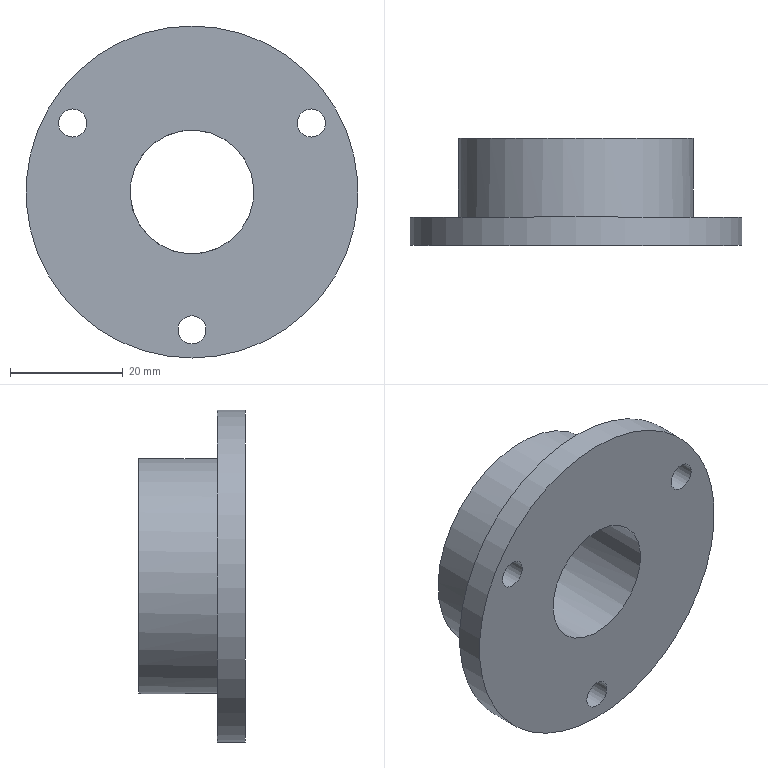Part | STEP file | YBQDJ-YB-12 | 1 solid | 11 faces | box 59 x 19 x 59 mm | volume 24092 mm3 | cylinder 7 | plane 4 | commonest cylinder face diameters 5 x3 22 x1 32 x1 41.8 x1 59 x1
STEP:
#1=CARTESIAN_POINT('',(0.,0.,0.));
#2=DIRECTION('',(0.,0.,1.));
#3=DIRECTION('',(1.,0.,0.));
#4=AXIS2_PLACEMENT_3D('',#1,#2,#3);
#5=CARTESIAN_POINT('',(-168.721,-300.,118.779));
#6=VERTEX_POINT('',#5);
#7=CARTESIAN_POINT('',(-183.5,-300.,104.));
#8=DIRECTION('',(0.,1.,0.));
#9=DIRECTION('',(0.7071,0.,0.7071));
#10=AXIS2_PLACEMENT_3D('',#7,#8,#9);
#11=CIRCLE('',#10,20.9);
#12=CARTESIAN_POINT('',(-183.5,-295.,104.));
#13=DIRECTION('',(0.,-1.,0.));
#14=DIRECTION('',(0.7071,0.,0.7071));
#15=AXIS2_PLACEMENT_3D('',#12,#13,#14);
#16=CYLINDRICAL_SURFACE('',#15,20.9);
#17=CARTESIAN_POINT('',(6.283,5.));
#18=DIRECTION('',(-1.,0.));
#19=VECTOR('',#18,1.);
#20=LINE('',#17,#19);
#21=(GEOMETRIC_REPRESENTATION_CONTEXT(2)PARAMETRIC_REPRESENTATION_CONTEXT()REPRESENTATION_CONTEXT('',''));
#22=DEFINITIONAL_REPRESENTATION('',(#20),#21);
#23=PCURVE('',#16,#22);
#24=CARTESIAN_POINT('',(-183.5,-300.,104.));
#25=DIRECTION('',(0.,1.,0.));
#26=DIRECTION('',(-0.7071,0.,-0.7071));
#27=AXIS2_PLACEMENT_3D('',#24,#25,#26);
#28=PLANE('',#27);
#29=CARTESIAN_POINT('',(0.,0.));
#30=DIRECTION('',(-1.,0.));
#31=AXIS2_PLACEMENT_2D('',#29,#30);
#32=CIRCLE('',#31,20.9);
#33=(GEOMETRIC_REPRESENTATION_CONTEXT(2)PARAMETRIC_REPRESENTATION_CONTEXT()REPRESENTATION_CONTEXT('',''));
#34=DEFINITIONAL_REPRESENTATION('',(#32),#33);
#35=PCURVE('',#28,#34);
#36=SURFACE_CURVE('',#11,(#23,#35),.PCURVE_S1.);
#37=EDGE_CURVE('',#6,#6,#36,.T.);
#38=ORIENTED_EDGE('',*,*,#37,.T.);
#39=CARTESIAN_POINT('',(-168.721,-286.,118.779));
#40=VERTEX_POINT('',#39);
#41=CARTESIAN_POINT('',(-168.721,-286.,118.779));
#42=CARTESIAN_POINT('',(-168.721,-300.,118.779));
#43=B_SPLINE_CURVE_WITH_KNOTS('',1,(#41,#42),.UNSPECIFIED.,.F.,.F.,(2,2),(-9.,5.),.PIECEWISE_BEZIER_KNOTS.);
#44=CARTESIAN_POINT('',(0.,0.));
#45=DIRECTION('',(0.,1.));
#46=VECTOR('',#45,1.);
#47=LINE('',#44,#46);
#48=(GEOMETRIC_REPRESENTATION_CONTEXT(2)PARAMETRIC_REPRESENTATION_CONTEXT()REPRESENTATION_CONTEXT('',''));
#49=DEFINITIONAL_REPRESENTATION('',(#47),#48);
#50=PCURVE('',#16,#49);
#51=CARTESIAN_POINT('',(6.283,0.));
#52=DIRECTION('',(0.,1.));
#53=VECTOR('',#52,1.);
#54=LINE('',#51,#53);
#55=(GEOMETRIC_REPRESENTATION_CONTEXT(2)PARAMETRIC_REPRESENTATION_CONTEXT()REPRESENTATION_CONTEXT('',''));
#56=DEFINITIONAL_REPRESENTATION('',(#54),#55);
#57=PCURVE('',#16,#56);
#58=SEAM_CURVE('',#43,(#50,#57),.PCURVE_S1.);
#59=EDGE_CURVE('',#40,#6,#58,.T.);
#60=ORIENTED_EDGE('',*,*,#59,.F.);
#61=CARTESIAN_POINT('',(-183.5,-286.,83.1));
#62=VERTEX_POINT('',#61);
#63=CARTESIAN_POINT('',(-183.5,-286.,104.));
#64=DIRECTION('',(0.,-1.,0.));
#65=DIRECTION('',(0.,0.,-1.));
#66=AXIS2_PLACEMENT_3D('',#63,#64,#65);
#67=CIRCLE('',#66,20.9);
#68=CARTESIAN_POINT('',(-2.356,-9.));
#69=DIRECTION('',(1.,0.));
#70=VECTOR('',#69,1.);
#71=LINE('',#68,#70);
#72=(GEOMETRIC_REPRESENTATION_CONTEXT(2)PARAMETRIC_REPRESENTATION_CONTEXT()REPRESENTATION_CONTEXT('',''));
#73=DEFINITIONAL_REPRESENTATION('',(#71),#72);
#74=PCURVE('',#16,#73);
#75=CARTESIAN_POINT('',(-183.5,-286.,94.));
#76=DIRECTION('',(0.,-1.,0.));
#77=DIRECTION('',(0.,0.,1.));
#78=AXIS2_PLACEMENT_3D('',#75,#76,#77);
#79=PLANE('',#78);
#80=CARTESIAN_POINT('',(10.,0.));
#81=DIRECTION('',(-1.,0.));
#82=AXIS2_PLACEMENT_2D('',#80,#81);
#83=CIRCLE('',#82,20.9);
#84=(GEOMETRIC_REPRESENTATION_CONTEXT(2)PARAMETRIC_REPRESENTATION_CONTEXT()REPRESENTATION_CONTEXT('',''));
#85=DEFINITIONAL_REPRESENTATION('',(#83),#84);
#86=PCURVE('',#79,#85);
#87=SURFACE_CURVE('',#67,(#74,#86),.PCURVE_S1.);
#88=EDGE_CURVE('',#40,#62,#87,.T.);
#89=ORIENTED_EDGE('',*,*,#88,.T.);
#90=CARTESIAN_POINT('',(-183.5,-286.,104.));
#91=DIRECTION('',(0.,-1.,0.));
#92=DIRECTION('',(0.,0.,-1.));
#93=AXIS2_PLACEMENT_3D('',#90,#91,#92);
#94=CIRCLE('',#93,20.9);
#95=CARTESIAN_POINT('',(3.927,-9.));
#96=DIRECTION('',(1.,0.));
#97=VECTOR('',#96,1.);
#98=LINE('',#95,#97);
#99=(GEOMETRIC_REPRESENTATION_CONTEXT(2)PARAMETRIC_REPRESENTATION_CONTEXT()REPRESENTATION_CONTEXT('',''));
#100=DEFINITIONAL_REPRESENTATION('',(#98),#99);
#101=PCURVE('',#16,#100);
#102=CARTESIAN_POINT('',(10.,0.));
#103=DIRECTION('',(-1.,0.));
#104=AXIS2_PLACEMENT_2D('',#102,#103);
#105=CIRCLE('',#104,20.9);
#106=(GEOMETRIC_REPRESENTATION_CONTEXT(2)PARAMETRIC_REPRESENTATION_CONTEXT()REPRESENTATION_CONTEXT('',''));
#107=DEFINITIONAL_REPRESENTATION('',(#105),#106);
#108=PCURVE('',#79,#107);
#109=SURFACE_CURVE('',#94,(#101,#108),.PCURVE_S1.);
#110=EDGE_CURVE('',#62,#40,#109,.T.);
#111=ORIENTED_EDGE('',*,*,#110,.T.);
#112=ORIENTED_EDGE('',*,*,#59,.T.);
#113=EDGE_LOOP('',(#38,#60,#89,#111,#112));
#114=FACE_BOUND('',#113,.T.);
#115=ADVANCED_FACE('',(#114),#16,.T.);
#116=CARTESIAN_POINT('',(-183.5,-305.,133.5));
#117=VERTEX_POINT('',#116);
#118=CARTESIAN_POINT('',(-183.5,-305.,104.));
#119=DIRECTION('',(0.,-1.,0.));
#120=DIRECTION('',(0.,0.,1.));
#121=AXIS2_PLACEMENT_3D('',#118,#119,#120);
#122=CIRCLE('',#121,29.5);
#123=CARTESIAN_POINT('',(-183.5,-305.,104.));
#124=DIRECTION('',(0.,1.,0.));
#125=DIRECTION('',(-0.7071,0.,-0.7071));
#126=AXIS2_PLACEMENT_3D('',#123,#124,#125);
#127=CYLINDRICAL_SURFACE('',#126,29.5);
#128=CARTESIAN_POINT('',(8.639,0.));
#129=DIRECTION('',(-1.,0.));
#130=VECTOR('',#129,1.);
#131=LINE('',#128,#130);
#132=(GEOMETRIC_REPRESENTATION_CONTEXT(2)PARAMETRIC_REPRESENTATION_CONTEXT()REPRESENTATION_CONTEXT('',''));
#133=DEFINITIONAL_REPRESENTATION('',(#131),#132);
#134=PCURVE('',#127,#133);
#135=CARTESIAN_POINT('',(-183.5,-305.,104.));
#136=DIRECTION('',(0.,1.,0.));
#137=DIRECTION('',(-0.7071,0.,-0.7071));
#138=AXIS2_PLACEMENT_3D('',#135,#136,#137);
#139=PLANE('',#138);
#140=CARTESIAN_POINT('',(-20.86,20.86));
#141=CARTESIAN_POINT('',(15.27,56.99));
#142=CARTESIAN_POINT('',(28.495,7.635));
#143=CARTESIAN_POINT('',(41.719,-41.719));
#144=CARTESIAN_POINT('',(-7.635,-28.495));
#145=CARTESIAN_POINT('',(-56.99,-15.27));
#146=CARTESIAN_POINT('',(-20.86,20.86));
#147=(BOUNDED_CURVE()B_SPLINE_CURVE(2,(#140,#141,#142,#143,#144,#145,#146),.UNSPECIFIED.,.T.,.F.)B_SPLINE_CURVE_WITH_KNOTS((1,2,2,2,2,1),(-2.094,0.,2.094,4.189,6.283,8.378),.UNSPECIFIED.)CURVE()GEOMETRIC_REPRESENTATION_ITEM()RATIONAL_B_SPLINE_CURVE((1.,0.5,1.,0.5,1.,0.5,1.))REPRESENTATION_ITEM(''));
#148=(GEOMETRIC_REPRESENTATION_CONTEXT(2)PARAMETRIC_REPRESENTATION_CONTEXT()REPRESENTATION_CONTEXT('',''));
#149=DEFINITIONAL_REPRESENTATION('',(#147),#148);
#150=PCURVE('',#139,#149);
#151=SURFACE_CURVE('',#122,(#134,#150),.PCURVE_S1.);
#152=EDGE_CURVE('',#117,#117,#151,.T.);
#153=ORIENTED_EDGE('',*,*,#152,.F.);
#154=CARTESIAN_POINT('',(-183.5,-300.,133.5));
#155=VERTEX_POINT('',#154);
#156=CARTESIAN_POINT('',(-183.5,-305.,133.5));
#157=CARTESIAN_POINT('',(-183.5,-300.,133.5));
#158=B_SPLINE_CURVE_WITH_KNOTS('',1,(#156,#157),.UNSPECIFIED.,.F.,.F.,(2,2),(0.,5.),.PIECEWISE_BEZIER_KNOTS.);
#159=CARTESIAN_POINT('',(8.639,0.));
#160=DIRECTION('',(0.,1.));
#161=VECTOR('',#160,1.);
#162=LINE('',#159,#161);
#163=(GEOMETRIC_REPRESENTATION_CONTEXT(2)PARAMETRIC_REPRESENTATION_CONTEXT()REPRESENTATION_CONTEXT('',''));
#164=DEFINITIONAL_REPRESENTATION('',(#162),#163);
#165=PCURVE('',#127,#164);
#166=CARTESIAN_POINT('',(2.356,0.));
#167=DIRECTION('',(0.,1.));
#168=VECTOR('',#167,1.);
#169=LINE('',#166,#168);
#170=(GEOMETRIC_REPRESENTATION_CONTEXT(2)PARAMETRIC_REPRESENTATION_CONTEXT()REPRESENTATION_CONTEXT('',''));
#171=DEFINITIONAL_REPRESENTATION('',(#169),#170);
#172=PCURVE('',#127,#171);
#173=SEAM_CURVE('',#158,(#165,#172),.PCURVE_S1.);
#174=EDGE_CURVE('',#117,#155,#173,.T.);
#175=ORIENTED_EDGE('',*,*,#174,.T.);
#176=CARTESIAN_POINT('',(-183.5,-300.,104.));
#177=DIRECTION('',(0.,-1.,0.));
#178=DIRECTION('',(0.,0.,1.));
#179=AXIS2_PLACEMENT_3D('',#176,#177,#178);
#180=CIRCLE('',#179,29.5);
#181=CARTESIAN_POINT('',(8.639,5.));
#182=DIRECTION('',(-1.,0.));
#183=VECTOR('',#182,1.);
#184=LINE('',#181,#183);
#185=(GEOMETRIC_REPRESENTATION_CONTEXT(2)PARAMETRIC_REPRESENTATION_CONTEXT()REPRESENTATION_CONTEXT('',''));
#186=DEFINITIONAL_REPRESENTATION('',(#184),#185);
#187=PCURVE('',#127,#186);
#188=CARTESIAN_POINT('',(-20.86,20.86));
#189=CARTESIAN_POINT('',(15.27,56.99));
#190=CARTESIAN_POINT('',(28.495,7.635));
#191=CARTESIAN_POINT('',(41.719,-41.719));
#192=CARTESIAN_POINT('',(-7.635,-28.495));
#193=CARTESIAN_POINT('',(-56.99,-15.27));
#194=CARTESIAN_POINT('',(-20.86,20.86));
#195=(BOUNDED_CURVE()B_SPLINE_CURVE(2,(#188,#189,#190,#191,#192,#193,#194),.UNSPECIFIED.,.T.,.F.)B_SPLINE_CURVE_WITH_KNOTS((1,2,2,2,2,1),(-2.094,0.,2.094,4.189,6.283,8.378),.UNSPECIFIED.)CURVE()GEOMETRIC_REPRESENTATION_ITEM()RATIONAL_B_SPLINE_CURVE((1.,0.5,1.,0.5,1.,0.5,1.))REPRESENTATION_ITEM(''));
#196=(GEOMETRIC_REPRESENTATION_CONTEXT(2)PARAMETRIC_REPRESENTATION_CONTEXT()REPRESENTATION_CONTEXT('',''));
#197=DEFINITIONAL_REPRESENTATION('',(#195),#196);
#198=PCURVE('',#28,#197);
#199=SURFACE_CURVE('',#180,(#187,#198),.PCURVE_S1.);
#200=EDGE_CURVE('',#155,#155,#199,.T.);
#201=ORIENTED_EDGE('',*,*,#200,.T.);
#202=ORIENTED_EDGE('',*,*,#174,.F.);
#203=EDGE_LOOP('',(#153,#175,#201,#202));
#204=FACE_BOUND('',#203,.T.);
#205=ADVANCED_FACE('',(#204),#127,.T.);
#206=CARTESIAN_POINT('',(-204.718,-305.,118.75));
#207=VERTEX_POINT('',#206);
#208=CARTESIAN_POINT('',(-204.718,-305.,116.25));
#209=DIRECTION('',(0.,-1.,0.));
#210=DIRECTION('',(0.,0.,1.));
#211=AXIS2_PLACEMENT_3D('',#208,#209,#210);
#212=CIRCLE('',#211,2.5);
#213=CARTESIAN_POINT('',(4.573,25.433));
#214=CARTESIAN_POINT('',(7.635,28.495));
#215=CARTESIAN_POINT('',(8.756,24.312));
#216=CARTESIAN_POINT('',(9.877,20.13));
#217=CARTESIAN_POINT('',(5.694,21.25));
#218=CARTESIAN_POINT('',(1.511,22.371));
#219=CARTESIAN_POINT('',(4.573,25.433));
#220=(BOUNDED_CURVE()B_SPLINE_CURVE(2,(#213,#214,#215,#216,#217,#218,#219),.UNSPECIFIED.,.T.,.F.)B_SPLINE_CURVE_WITH_KNOTS((1,2,2,2,2,1),(-2.094,0.,2.094,4.189,6.283,8.378),.UNSPECIFIED.)CURVE()GEOMETRIC_REPRESENTATION_ITEM()RATIONAL_B_SPLINE_CURVE((1.,0.5,1.,0.5,1.,0.5,1.))REPRESENTATION_ITEM(''));
#221=(GEOMETRIC_REPRESENTATION_CONTEXT(2)PARAMETRIC_REPRESENTATION_CONTEXT()REPRESENTATION_CONTEXT('',''));
#222=DEFINITIONAL_REPRESENTATION('',(#220),#221);
#223=PCURVE('',#139,#222);
#224=CARTESIAN_POINT('',(-204.718,-292.8,116.25));
#225=DIRECTION('',(0.,-1.,0.));
#226=DIRECTION('',(1.,0.,0.));
#227=AXIS2_PLACEMENT_3D('',#224,#225,#226);
#228=CYLINDRICAL_SURFACE('',#227,2.5);
#229=CARTESIAN_POINT('',(1.571,12.2));
#230=DIRECTION('',(1.,0.));
#231=VECTOR('',#230,1.);
#232=LINE('',#229,#231);
#233=(GEOMETRIC_REPRESENTATION_CONTEXT(2)PARAMETRIC_REPRESENTATION_CONTEXT()REPRESENTATION_CONTEXT('',''));
#234=DEFINITIONAL_REPRESENTATION('',(#232),#233);
#235=PCURVE('',#228,#234);
#236=SURFACE_CURVE('',#212,(#223,#235),.PCURVE_S1.);
#237=EDGE_CURVE('',#207,#207,#236,.T.);
#238=ORIENTED_EDGE('',*,*,#237,.F.);
#239=EDGE_LOOP('',(#238));
#240=FACE_BOUND('',#239,.T.);
#241=CARTESIAN_POINT('',(-183.5,-305.,82.));
#242=VERTEX_POINT('',#241);
#243=CARTESIAN_POINT('',(-183.5,-305.,79.5));
#244=DIRECTION('',(0.,-1.,0.));
#245=DIRECTION('',(0.,0.,1.));
#246=AXIS2_PLACEMENT_3D('',#243,#244,#245);
#247=CIRCLE('',#246,2.5);
#248=CARTESIAN_POINT('',(15.556,-15.556));
#249=CARTESIAN_POINT('',(18.618,-12.494));
#250=CARTESIAN_POINT('',(19.739,-16.677));
#251=CARTESIAN_POINT('',(20.86,-20.86));
#252=CARTESIAN_POINT('',(16.677,-19.739));
#253=CARTESIAN_POINT('',(12.494,-18.618));
#254=CARTESIAN_POINT('',(15.556,-15.556));
#255=(BOUNDED_CURVE()B_SPLINE_CURVE(2,(#248,#249,#250,#251,#252,#253,#254),.UNSPECIFIED.,.T.,.F.)B_SPLINE_CURVE_WITH_KNOTS((1,2,2,2,2,1),(-2.094,0.,2.094,4.189,6.283,8.378),.UNSPECIFIED.)CURVE()GEOMETRIC_REPRESENTATION_ITEM()RATIONAL_B_SPLINE_CURVE((1.,0.5,1.,0.5,1.,0.5,1.))REPRESENTATION_ITEM(''));
#256=(GEOMETRIC_REPRESENTATION_CONTEXT(2)PARAMETRIC_REPRESENTATION_CONTEXT()REPRESENTATION_CONTEXT('',''));
#257=DEFINITIONAL_REPRESENTATION('',(#255),#256);
#258=PCURVE('',#139,#257);
#259=CARTESIAN_POINT('',(-183.5,-292.8,79.5));
#260=DIRECTION('',(0.,-1.,0.));
#261=DIRECTION('',(1.,0.,0.));
#262=AXIS2_PLACEMENT_3D('',#259,#260,#261);
#263=CYLINDRICAL_SURFACE('',#262,2.5);
#264=CARTESIAN_POINT('',(1.571,12.2));
#265=DIRECTION('',(1.,0.));
#266=VECTOR('',#265,1.);
#267=LINE('',#264,#266);
#268=(GEOMETRIC_REPRESENTATION_CONTEXT(2)PARAMETRIC_REPRESENTATION_CONTEXT()REPRESENTATION_CONTEXT('',''));
#269=DEFINITIONAL_REPRESENTATION('',(#267),#268);
#270=PCURVE('',#263,#269);
#271=SURFACE_CURVE('',#247,(#258,#270),.PCURVE_S1.);
#272=EDGE_CURVE('',#242,#242,#271,.T.);
#273=ORIENTED_EDGE('',*,*,#272,.F.);
#274=EDGE_LOOP('',(#273));
#275=FACE_BOUND('',#274,.T.);
#276=CARTESIAN_POINT('',(-162.282,-305.,118.75));
#277=VERTEX_POINT('',#276);
#278=CARTESIAN_POINT('',(-162.282,-305.,116.25));
#279=DIRECTION('',(0.,-1.,0.));
#280=DIRECTION('',(0.,0.,1.));
#281=AXIS2_PLACEMENT_3D('',#278,#279,#280);
#282=CIRCLE('',#281,2.5);
#283=CARTESIAN_POINT('',(-25.433,-4.573));
#284=CARTESIAN_POINT('',(-22.371,-1.511));
#285=CARTESIAN_POINT('',(-21.25,-5.694));
#286=CARTESIAN_POINT('',(-20.13,-9.877));
#287=CARTESIAN_POINT('',(-24.312,-8.756));
#288=CARTESIAN_POINT('',(-28.495,-7.635));
#289=CARTESIAN_POINT('',(-25.433,-4.573));
#290=(BOUNDED_CURVE()B_SPLINE_CURVE(2,(#283,#284,#285,#286,#287,#288,#289),.UNSPECIFIED.,.T.,.F.)B_SPLINE_CURVE_WITH_KNOTS((1,2,2,2,2,1),(-2.094,0.,2.094,4.189,6.283,8.378),.UNSPECIFIED.)CURVE()GEOMETRIC_REPRESENTATION_ITEM()RATIONAL_B_SPLINE_CURVE((1.,0.5,1.,0.5,1.,0.5,1.))REPRESENTATION_ITEM(''));
#291=(GEOMETRIC_REPRESENTATION_CONTEXT(2)PARAMETRIC_REPRESENTATION_CONTEXT()REPRESENTATION_CONTEXT('',''));
#292=DEFINITIONAL_REPRESENTATION('',(#290),#291);
#293=PCURVE('',#139,#292);
#294=CARTESIAN_POINT('',(-162.282,-292.8,116.25));
#295=DIRECTION('',(0.,-1.,0.));
#296=DIRECTION('',(1.,0.,0.));
#297=AXIS2_PLACEMENT_3D('',#294,#295,#296);
#298=CYLINDRICAL_SURFACE('',#297,2.5);
#299=CARTESIAN_POINT('',(1.571,12.2));
#300=DIRECTION('',(1.,0.));
#301=VECTOR('',#300,1.);
#302=LINE('',#299,#301);
#303=(GEOMETRIC_REPRESENTATION_CONTEXT(2)PARAMETRIC_REPRESENTATION_CONTEXT()REPRESENTATION_CONTEXT('',''));
#304=DEFINITIONAL_REPRESENTATION('',(#302),#303);
#305=PCURVE('',#298,#304);
#306=SURFACE_CURVE('',#282,(#293,#305),.PCURVE_S1.);
#307=EDGE_CURVE('',#277,#277,#306,.T.);
#308=ORIENTED_EDGE('',*,*,#307,.F.);
#309=EDGE_LOOP('',(#308));
#310=FACE_BOUND('',#309,.T.);
#311=ORIENTED_EDGE('',*,*,#152,.T.);
#312=EDGE_LOOP('',(#311));
#313=FACE_BOUND('',#312,.T.);
#314=CARTESIAN_POINT('',(-175.722,-305.,111.778));
#315=VERTEX_POINT('',#314);
#316=CARTESIAN_POINT('',(-183.5,-305.,104.));
#317=DIRECTION('',(0.,1.,0.));
#318=DIRECTION('',(0.7071,0.,0.7071));
#319=AXIS2_PLACEMENT_3D('',#316,#317,#318);
#320=CIRCLE('',#319,11.);
#321=CARTESIAN_POINT('',(0.,0.));
#322=DIRECTION('',(-1.,0.));
#323=AXIS2_PLACEMENT_2D('',#321,#322);
#324=CIRCLE('',#323,11.);
#325=(GEOMETRIC_REPRESENTATION_CONTEXT(2)PARAMETRIC_REPRESENTATION_CONTEXT()REPRESENTATION_CONTEXT('',''));
#326=DEFINITIONAL_REPRESENTATION('',(#324),#325);
#327=PCURVE('',#139,#326);
#328=CARTESIAN_POINT('',(-183.5,-295.,104.));
#329=DIRECTION('',(0.,-1.,0.));
#330=DIRECTION('',(0.7071,0.,0.7071));
#331=AXIS2_PLACEMENT_3D('',#328,#329,#330);
#332=CYLINDRICAL_SURFACE('',#331,11.);
#333=CARTESIAN_POINT('',(6.283,10.));
#334=DIRECTION('',(-1.,0.));
#335=VECTOR('',#334,1.);
#336=LINE('',#333,#335);
#337=(GEOMETRIC_REPRESENTATION_CONTEXT(2)PARAMETRIC_REPRESENTATION_CONTEXT()REPRESENTATION_CONTEXT('',''));
#338=DEFINITIONAL_REPRESENTATION('',(#336),#337);
#339=PCURVE('',#332,#338);
#340=SURFACE_CURVE('',#320,(#327,#339),.PCURVE_S1.);
#341=EDGE_CURVE('',#315,#315,#340,.T.);
#342=ORIENTED_EDGE('',*,*,#341,.T.);
#343=EDGE_LOOP('',(#342));
#344=FACE_BOUND('',#343,.T.);
#345=ADVANCED_FACE('',(#240,#275,#310,#313,#344),#139,.F.);
#346=CARTESIAN_POINT('',(-204.718,-300.,118.75));
#347=VERTEX_POINT('',#346);
#348=CARTESIAN_POINT('',(-204.718,-300.,116.25));
#349=DIRECTION('',(0.,-1.,0.));
#350=DIRECTION('',(0.,0.,1.));
#351=AXIS2_PLACEMENT_3D('',#348,#349,#350);
#352=CIRCLE('',#351,2.5);
#353=CARTESIAN_POINT('',(4.573,25.433));
#354=CARTESIAN_POINT('',(7.635,28.495));
#355=CARTESIAN_POINT('',(8.756,24.312));
#356=CARTESIAN_POINT('',(9.877,20.13));
#357=CARTESIAN_POINT('',(5.694,21.25));
#358=CARTESIAN_POINT('',(1.511,22.371));
#359=CARTESIAN_POINT('',(4.573,25.433));
#360=(BOUNDED_CURVE()B_SPLINE_CURVE(2,(#353,#354,#355,#356,#357,#358,#359),.UNSPECIFIED.,.T.,.F.)B_SPLINE_CURVE_WITH_KNOTS((1,2,2,2,2,1),(-2.094,0.,2.094,4.189,6.283,8.378),.UNSPECIFIED.)CURVE()GEOMETRIC_REPRESENTATION_ITEM()RATIONAL_B_SPLINE_CURVE((1.,0.5,1.,0.5,1.,0.5,1.))REPRESENTATION_ITEM(''));
#361=(GEOMETRIC_REPRESENTATION_CONTEXT(2)PARAMETRIC_REPRESENTATION_CONTEXT()REPRESENTATION_CONTEXT('',''));
#362=DEFINITIONAL_REPRESENTATION('',(#360),#361);
#363=PCURVE('',#28,#362);
#364=CARTESIAN_POINT('',(1.571,7.2));
#365=DIRECTION('',(1.,0.));
#366=VECTOR('',#365,1.);
#367=LINE('',#364,#366);
#368=(GEOMETRIC_REPRESENTATION_CONTEXT(2)PARAMETRIC_REPRESENTATION_CONTEXT()REPRESENTATION_CONTEXT('',''));
#369=DEFINITIONAL_REPRESENTATION('',(#367),#368);
#370=PCURVE('',#228,#369);
#371=SURFACE_CURVE('',#352,(#363,#370),.PCURVE_S1.);
#372=EDGE_CURVE('',#347,#347,#371,.T.);
#373=ORIENTED_EDGE('',*,*,#372,.T.);
#374=EDGE_LOOP('',(#373));
#375=FACE_BOUND('',#374,.T.);
#376=CARTESIAN_POINT('',(-183.5,-300.,82.));
#377=VERTEX_POINT('',#376);
#378=CARTESIAN_POINT('',(-183.5,-300.,79.5));
#379=DIRECTION('',(0.,-1.,0.));
#380=DIRECTION('',(0.,0.,1.));
#381=AXIS2_PLACEMENT_3D('',#378,#379,#380);
#382=CIRCLE('',#381,2.5);
#383=CARTESIAN_POINT('',(15.556,-15.556));
#384=CARTESIAN_POINT('',(18.618,-12.494));
#385=CARTESIAN_POINT('',(19.739,-16.677));
#386=CARTESIAN_POINT('',(20.86,-20.86));
#387=CARTESIAN_POINT('',(16.677,-19.739));
#388=CARTESIAN_POINT('',(12.494,-18.618));
#389=CARTESIAN_POINT('',(15.556,-15.556));
#390=(BOUNDED_CURVE()B_SPLINE_CURVE(2,(#383,#384,#385,#386,#387,#388,#389),.UNSPECIFIED.,.T.,.F.)B_SPLINE_CURVE_WITH_KNOTS((1,2,2,2,2,1),(-2.094,0.,2.094,4.189,6.283,8.378),.UNSPECIFIED.)CURVE()GEOMETRIC_REPRESENTATION_ITEM()RATIONAL_B_SPLINE_CURVE((1.,0.5,1.,0.5,1.,0.5,1.))REPRESENTATION_ITEM(''));
#391=(GEOMETRIC_REPRESENTATION_CONTEXT(2)PARAMETRIC_REPRESENTATION_CONTEXT()REPRESENTATION_CONTEXT('',''));
#392=DEFINITIONAL_REPRESENTATION('',(#390),#391);
#393=PCURVE('',#28,#392);
#394=CARTESIAN_POINT('',(1.571,7.2));
#395=DIRECTION('',(1.,0.));
#396=VECTOR('',#395,1.);
#397=LINE('',#394,#396);
#398=(GEOMETRIC_REPRESENTATION_CONTEXT(2)PARAMETRIC_REPRESENTATION_CONTEXT()REPRESENTATION_CONTEXT('',''));
#399=DEFINITIONAL_REPRESENTATION('',(#397),#398);
#400=PCURVE('',#263,#399);
#401=SURFACE_CURVE('',#382,(#393,#400),.PCURVE_S1.);
#402=EDGE_CURVE('',#377,#377,#401,.T.);
#403=ORIENTED_EDGE('',*,*,#402,.T.);
#404=EDGE_LOOP('',(#403));
#405=FACE_BOUND('',#404,.T.);
#406=CARTESIAN_POINT('',(-162.282,-300.,118.75));
#407=VERTEX_POINT('',#406);
#408=CARTESIAN_POINT('',(-162.282,-300.,116.25));
#409=DIRECTION('',(0.,-1.,0.));
#410=DIRECTION('',(0.,0.,1.));
#411=AXIS2_PLACEMENT_3D('',#408,#409,#410);
#412=CIRCLE('',#411,2.5);
#413=CARTESIAN_POINT('',(-25.433,-4.573));
#414=CARTESIAN_POINT('',(-22.371,-1.511));
#415=CARTESIAN_POINT('',(-21.25,-5.694));
#416=CARTESIAN_POINT('',(-20.13,-9.877));
#417=CARTESIAN_POINT('',(-24.312,-8.756));
#418=CARTESIAN_POINT('',(-28.495,-7.635));
#419=CARTESIAN_POINT('',(-25.433,-4.573));
#420=(BOUNDED_CURVE()B_SPLINE_CURVE(2,(#413,#414,#415,#416,#417,#418,#419),.UNSPECIFIED.,.T.,.F.)B_SPLINE_CURVE_WITH_KNOTS((1,2,2,2,2,1),(-2.094,0.,2.094,4.189,6.283,8.378),.UNSPECIFIED.)CURVE()GEOMETRIC_REPRESENTATION_ITEM()RATIONAL_B_SPLINE_CURVE((1.,0.5,1.,0.5,1.,0.5,1.))REPRESENTATION_ITEM(''));
#421=(GEOMETRIC_REPRESENTATION_CONTEXT(2)PARAMETRIC_REPRESENTATION_CONTEXT()REPRESENTATION_CONTEXT('',''));
#422=DEFINITIONAL_REPRESENTATION('',(#420),#421);
#423=PCURVE('',#28,#422);
#424=CARTESIAN_POINT('',(1.571,7.2));
#425=DIRECTION('',(1.,0.));
#426=VECTOR('',#425,1.);
#427=LINE('',#424,#426);
#428=(GEOMETRIC_REPRESENTATION_CONTEXT(2)PARAMETRIC_REPRESENTATION_CONTEXT()REPRESENTATION_CONTEXT('',''));
#429=DEFINITIONAL_REPRESENTATION('',(#427),#428);
#430=PCURVE('',#298,#429);
#431=SURFACE_CURVE('',#412,(#423,#430),.PCURVE_S1.);
#432=EDGE_CURVE('',#407,#407,#431,.T.);
#433=ORIENTED_EDGE('',*,*,#432,.T.);
#434=EDGE_LOOP('',(#433));
#435=FACE_BOUND('',#434,.T.);
#436=ORIENTED_EDGE('',*,*,#200,.F.);
#437=EDGE_LOOP('',(#436));
#438=FACE_BOUND('',#437,.T.);
#439=ORIENTED_EDGE('',*,*,#37,.F.);
#440=EDGE_LOOP('',(#439));
#441=FACE_BOUND('',#440,.T.);
#442=ADVANCED_FACE('',(#375,#405,#435,#438,#441),#28,.T.);
#443=CARTESIAN_POINT('',(-183.5,-286.,88.));
#444=VERTEX_POINT('',#443);
#445=CARTESIAN_POINT('',(-183.5,-286.,104.));
#446=DIRECTION('',(0.,-1.,0.));
#447=DIRECTION('',(0.,0.,-1.));
#448=AXIS2_PLACEMENT_3D('',#445,#446,#447);
#449=CIRCLE('',#448,16.);
#450=CARTESIAN_POINT('',(10.,0.));
#451=DIRECTION('',(-1.,0.));
#452=AXIS2_PLACEMENT_2D('',#450,#451);
#453=CIRCLE('',#452,16.);
#454=(GEOMETRIC_REPRESENTATION_CONTEXT(2)PARAMETRIC_REPRESENTATION_CONTEXT()REPRESENTATION_CONTEXT('',''));
#455=DEFINITIONAL_REPRESENTATION('',(#453),#454);
#456=PCURVE('',#79,#455);
#457=CARTESIAN_POINT('',(-183.5,-286.,104.));
#458=DIRECTION('',(0.,-1.,0.));
#459=DIRECTION('',(1.,0.,0.));
#460=AXIS2_PLACEMENT_3D('',#457,#458,#459);
#461=CYLINDRICAL_SURFACE('',#460,16.);
#462=CARTESIAN_POINT('',(4.712,0.));
#463=DIRECTION('',(1.,0.));
#464=VECTOR('',#463,1.);
#465=LINE('',#462,#464);
#466=(GEOMETRIC_REPRESENTATION_CONTEXT(2)PARAMETRIC_REPRESENTATION_CONTEXT()REPRESENTATION_CONTEXT('',''));
#467=DEFINITIONAL_REPRESENTATION('',(#465),#466);
#468=PCURVE('',#461,#467);
#469=SURFACE_CURVE('',#449,(#456,#468),.PCURVE_S1.);
#470=EDGE_CURVE('',#444,#444,#469,.T.);
#471=ORIENTED_EDGE('',*,*,#470,.T.);
#472=EDGE_LOOP('',(#471));
#473=FACE_BOUND('',#472,.T.);
#474=ORIENTED_EDGE('',*,*,#110,.F.);
#475=ORIENTED_EDGE('',*,*,#88,.F.);
#476=EDGE_LOOP('',(#474,#475));
#477=FACE_BOUND('',#476,.T.);
#478=ADVANCED_FACE('',(#473,#477),#79,.F.);
#479=CARTESIAN_POINT('',(-175.722,-289.,111.778));
#480=VERTEX_POINT('',#479);
#481=CARTESIAN_POINT('',(-183.5,-289.,93.));
#482=VERTEX_POINT('',#481);
#483=CARTESIAN_POINT('',(-183.5,-289.,104.));
#484=DIRECTION('',(0.,1.,0.));
#485=DIRECTION('',(0.,0.,-1.));
#486=AXIS2_PLACEMENT_3D('',#483,#484,#485);
#487=CIRCLE('',#486,11.);
#488=CARTESIAN_POINT('',(10.21,-6.));
#489=DIRECTION('',(-1.,0.));
#490=VECTOR('',#489,1.);
#491=LINE('',#488,#490);
#492=(GEOMETRIC_REPRESENTATION_CONTEXT(2)PARAMETRIC_REPRESENTATION_CONTEXT()REPRESENTATION_CONTEXT('',''));
#493=DEFINITIONAL_REPRESENTATION('',(#491),#492);
#494=PCURVE('',#332,#493);
#495=CARTESIAN_POINT('',(-183.5,-289.,104.));
#496=DIRECTION('',(0.,-1.,0.));
#497=DIRECTION('',(0.,0.,-1.));
#498=AXIS2_PLACEMENT_3D('',#495,#496,#497);
#499=PLANE('',#498);
#500=CARTESIAN_POINT('',(11.,0.));
#501=CARTESIAN_POINT('',(11.,-19.053));
#502=CARTESIAN_POINT('',(-5.5,-9.526));
#503=CARTESIAN_POINT('',(-22.,0.));
#504=CARTESIAN_POINT('',(-5.5,9.526));
#505=CARTESIAN_POINT('',(11.,19.053));
#506=CARTESIAN_POINT('',(11.,0.));
#507=(BOUNDED_CURVE()B_SPLINE_CURVE(2,(#500,#501,#502,#503,#504,#505,#506),.UNSPECIFIED.,.T.,.F.)B_SPLINE_CURVE_WITH_KNOTS((1,2,2,2,2,1),(-2.094,0.,2.094,4.189,6.283,8.378),.UNSPECIFIED.)CURVE()GEOMETRIC_REPRESENTATION_ITEM()RATIONAL_B_SPLINE_CURVE((1.,0.5,1.,0.5,1.,0.5,1.))REPRESENTATION_ITEM(''));
#508=(GEOMETRIC_REPRESENTATION_CONTEXT(2)PARAMETRIC_REPRESENTATION_CONTEXT()REPRESENTATION_CONTEXT('',''));
#509=DEFINITIONAL_REPRESENTATION('',(#507),#508);
#510=PCURVE('',#499,#509);
#511=SURFACE_CURVE('',#487,(#494,#510),.PCURVE_S1.);
#512=EDGE_CURVE('',#480,#482,#511,.T.);
#513=ORIENTED_EDGE('',*,*,#512,.F.);
#514=CARTESIAN_POINT('',(-175.722,-289.,111.778));
#515=CARTESIAN_POINT('',(-175.722,-305.,111.778));
#516=B_SPLINE_CURVE_WITH_KNOTS('',1,(#514,#515),.UNSPECIFIED.,.F.,.F.,(2,2),(-6.,10.),.PIECEWISE_BEZIER_KNOTS.);
#517=CARTESIAN_POINT('',(6.283,0.));
#518=DIRECTION('',(0.,1.));
#519=VECTOR('',#518,1.);
#520=LINE('',#517,#519);
#521=(GEOMETRIC_REPRESENTATION_CONTEXT(2)PARAMETRIC_REPRESENTATION_CONTEXT()REPRESENTATION_CONTEXT('',''));
#522=DEFINITIONAL_REPRESENTATION('',(#520),#521);
#523=PCURVE('',#332,#522);
#524=CARTESIAN_POINT('',(0.,0.));
#525=DIRECTION('',(0.,1.));
#526=VECTOR('',#525,1.);
#527=LINE('',#524,#526);
#528=(GEOMETRIC_REPRESENTATION_CONTEXT(2)PARAMETRIC_REPRESENTATION_CONTEXT()REPRESENTATION_CONTEXT('',''));
#529=DEFINITIONAL_REPRESENTATION('',(#527),#528);
#530=PCURVE('',#332,#529);
#531=SEAM_CURVE('',#516,(#523,#530),.PCURVE_S1.);
#532=EDGE_CURVE('',#480,#315,#531,.T.);
#533=ORIENTED_EDGE('',*,*,#532,.T.);
#534=ORIENTED_EDGE('',*,*,#341,.T.);
#535=ORIENTED_EDGE('',*,*,#532,.F.);
#536=CARTESIAN_POINT('',(-183.5,-289.,104.));
#537=DIRECTION('',(0.,1.,0.));
#538=DIRECTION('',(0.,0.,-1.));
#539=AXIS2_PLACEMENT_3D('',#536,#537,#538);
#540=CIRCLE('',#539,11.);
#541=CARTESIAN_POINT('',(3.927,-6.));
#542=DIRECTION('',(-1.,0.));
#543=VECTOR('',#542,1.);
#544=LINE('',#541,#543);
#545=(GEOMETRIC_REPRESENTATION_CONTEXT(2)PARAMETRIC_REPRESENTATION_CONTEXT()REPRESENTATION_CONTEXT('',''));
#546=DEFINITIONAL_REPRESENTATION('',(#544),#545);
#547=PCURVE('',#332,#546);
#548=CARTESIAN_POINT('',(11.,0.));
#549=CARTESIAN_POINT('',(11.,-19.053));
#550=CARTESIAN_POINT('',(-5.5,-9.526));
#551=CARTESIAN_POINT('',(-22.,0.));
#552=CARTESIAN_POINT('',(-5.5,9.526));
#553=CARTESIAN_POINT('',(11.,19.053));
#554=CARTESIAN_POINT('',(11.,0.));
#555=(BOUNDED_CURVE()B_SPLINE_CURVE(2,(#548,#549,#550,#551,#552,#553,#554),.UNSPECIFIED.,.T.,.F.)B_SPLINE_CURVE_WITH_KNOTS((1,2,2,2,2,1),(-2.094,0.,2.094,4.189,6.283,8.378),.UNSPECIFIED.)CURVE()GEOMETRIC_REPRESENTATION_ITEM()RATIONAL_B_SPLINE_CURVE((1.,0.5,1.,0.5,1.,0.5,1.))REPRESENTATION_ITEM(''));
#556=(GEOMETRIC_REPRESENTATION_CONTEXT(2)PARAMETRIC_REPRESENTATION_CONTEXT()REPRESENTATION_CONTEXT('',''));
#557=DEFINITIONAL_REPRESENTATION('',(#555),#556);
#558=PCURVE('',#499,#557);
#559=SURFACE_CURVE('',#540,(#547,#558),.PCURVE_S1.);
#560=EDGE_CURVE('',#482,#480,#559,.T.);
#561=ORIENTED_EDGE('',*,*,#560,.F.);
#562=EDGE_LOOP('',(#513,#533,#534,#535,#561));
#563=FACE_BOUND('',#562,.F.);
#564=ADVANCED_FACE('',(#563),#332,.F.);
#565=CARTESIAN_POINT('',(-183.5,-289.,88.));
#566=VERTEX_POINT('',#565);
#567=CARTESIAN_POINT('',(-183.5,-289.,104.));
#568=DIRECTION('',(0.,-1.,0.));
#569=DIRECTION('',(0.,0.,-1.));
#570=AXIS2_PLACEMENT_3D('',#567,#568,#569);
#571=CIRCLE('',#570,16.);
#572=CARTESIAN_POINT('',(0.,0.));
#573=DIRECTION('',(1.,0.));
#574=AXIS2_PLACEMENT_2D('',#572,#573);
#575=CIRCLE('',#574,16.);
#576=(GEOMETRIC_REPRESENTATION_CONTEXT(2)PARAMETRIC_REPRESENTATION_CONTEXT()REPRESENTATION_CONTEXT('',''));
#577=DEFINITIONAL_REPRESENTATION('',(#575),#576);
#578=PCURVE('',#499,#577);
#579=CARTESIAN_POINT('',(4.712,3.));
#580=DIRECTION('',(1.,0.));
#581=VECTOR('',#580,1.);
#582=LINE('',#579,#581);
#583=(GEOMETRIC_REPRESENTATION_CONTEXT(2)PARAMETRIC_REPRESENTATION_CONTEXT()REPRESENTATION_CONTEXT('',''));
#584=DEFINITIONAL_REPRESENTATION('',(#582),#583);
#585=PCURVE('',#461,#584);
#586=SURFACE_CURVE('',#571,(#578,#585),.PCURVE_S1.);
#587=EDGE_CURVE('',#566,#566,#586,.T.);
#588=ORIENTED_EDGE('',*,*,#587,.F.);
#589=EDGE_LOOP('',(#588));
#590=FACE_BOUND('',#589,.T.);
#591=ORIENTED_EDGE('',*,*,#560,.F.);
#592=ORIENTED_EDGE('',*,*,#512,.F.);
#593=EDGE_LOOP('',(#591,#592));
#594=FACE_BOUND('',#593,.T.);
#595=ADVANCED_FACE('',(#590,#594),#499,.F.);
#596=ORIENTED_EDGE('',*,*,#587,.F.);
#597=CARTESIAN_POINT('',(-183.5,-286.,88.));
#598=CARTESIAN_POINT('',(-183.5,-289.,88.));
#599=B_SPLINE_CURVE_WITH_KNOTS('',1,(#597,#598),.UNSPECIFIED.,.F.,.F.,(2,2),(0.,3.),.PIECEWISE_BEZIER_KNOTS.);
#600=CARTESIAN_POINT('',(4.712,0.));
#601=DIRECTION('',(0.,1.));
#602=VECTOR('',#601,1.);
#603=LINE('',#600,#602);
#604=(GEOMETRIC_REPRESENTATION_CONTEXT(2)PARAMETRIC_REPRESENTATION_CONTEXT()REPRESENTATION_CONTEXT('',''));
#605=DEFINITIONAL_REPRESENTATION('',(#603),#604);
#606=PCURVE('',#461,#605);
#607=CARTESIAN_POINT('',(10.996,0.));
#608=DIRECTION('',(0.,1.));
#609=VECTOR('',#608,1.);
#610=LINE('',#607,#609);
#611=(GEOMETRIC_REPRESENTATION_CONTEXT(2)PARAMETRIC_REPRESENTATION_CONTEXT()REPRESENTATION_CONTEXT('',''));
#612=DEFINITIONAL_REPRESENTATION('',(#610),#611);
#613=PCURVE('',#461,#612);
#614=SEAM_CURVE('',#599,(#606,#613),.PCURVE_S1.);
#615=EDGE_CURVE('',#444,#566,#614,.T.);
#616=ORIENTED_EDGE('',*,*,#615,.F.);
#617=ORIENTED_EDGE('',*,*,#470,.T.);
#618=ORIENTED_EDGE('',*,*,#615,.T.);
#619=EDGE_LOOP('',(#596,#616,#617,#618));
#620=FACE_BOUND('',#619,.F.);
#621=ADVANCED_FACE('',(#620),#461,.F.);
#622=ORIENTED_EDGE('',*,*,#432,.T.);
#623=CARTESIAN_POINT('',(-162.282,-300.,118.75));
#624=CARTESIAN_POINT('',(-162.282,-305.,118.75));
#625=B_SPLINE_CURVE_WITH_KNOTS('',1,(#623,#624),.UNSPECIFIED.,.F.,.F.,(2,2),(7.2,12.2),.PIECEWISE_BEZIER_KNOTS.);
#626=CARTESIAN_POINT('',(7.854,0.));
#627=DIRECTION('',(0.,1.));
#628=VECTOR('',#627,1.);
#629=LINE('',#626,#628);
#630=(GEOMETRIC_REPRESENTATION_CONTEXT(2)PARAMETRIC_REPRESENTATION_CONTEXT()REPRESENTATION_CONTEXT('',''));
#631=DEFINITIONAL_REPRESENTATION('',(#629),#630);
#632=PCURVE('',#298,#631);
#633=CARTESIAN_POINT('',(1.571,0.));
#634=DIRECTION('',(0.,1.));
#635=VECTOR('',#634,1.);
#636=LINE('',#633,#635);
#637=(GEOMETRIC_REPRESENTATION_CONTEXT(2)PARAMETRIC_REPRESENTATION_CONTEXT()REPRESENTATION_CONTEXT('',''));
#638=DEFINITIONAL_REPRESENTATION('',(#636),#637);
#639=PCURVE('',#298,#638);
#640=SEAM_CURVE('',#625,(#632,#639),.PCURVE_S1.);
#641=EDGE_CURVE('',#407,#277,#640,.T.);
#642=ORIENTED_EDGE('',*,*,#641,.T.);
#643=ORIENTED_EDGE('',*,*,#307,.F.);
#644=ORIENTED_EDGE('',*,*,#641,.F.);
#645=EDGE_LOOP('',(#622,#642,#643,#644));
#646=FACE_BOUND('',#645,.F.);
#647=ADVANCED_FACE('',(#646),#298,.F.);
#648=ORIENTED_EDGE('',*,*,#402,.T.);
#649=CARTESIAN_POINT('',(-183.5,-300.,82.));
#650=CARTESIAN_POINT('',(-183.5,-305.,82.));
#651=B_SPLINE_CURVE_WITH_KNOTS('',1,(#649,#650),.UNSPECIFIED.,.F.,.F.,(2,2),(7.2,12.2),.PIECEWISE_BEZIER_KNOTS.);
#652=CARTESIAN_POINT('',(7.854,0.));
#653=DIRECTION('',(0.,1.));
#654=VECTOR('',#653,1.);
#655=LINE('',#652,#654);
#656=(GEOMETRIC_REPRESENTATION_CONTEXT(2)PARAMETRIC_REPRESENTATION_CONTEXT()REPRESENTATION_CONTEXT('',''));
#657=DEFINITIONAL_REPRESENTATION('',(#655),#656);
#658=PCURVE('',#263,#657);
#659=CARTESIAN_POINT('',(1.571,0.));
#660=DIRECTION('',(0.,1.));
#661=VECTOR('',#660,1.);
#662=LINE('',#659,#661);
#663=(GEOMETRIC_REPRESENTATION_CONTEXT(2)PARAMETRIC_REPRESENTATION_CONTEXT()REPRESENTATION_CONTEXT('',''));
#664=DEFINITIONAL_REPRESENTATION('',(#662),#663);
#665=PCURVE('',#263,#664);
#666=SEAM_CURVE('',#651,(#658,#665),.PCURVE_S1.);
#667=EDGE_CURVE('',#377,#242,#666,.T.);
#668=ORIENTED_EDGE('',*,*,#667,.T.);
#669=ORIENTED_EDGE('',*,*,#272,.F.);
#670=ORIENTED_EDGE('',*,*,#667,.F.);
#671=EDGE_LOOP('',(#648,#668,#669,#670));
#672=FACE_BOUND('',#671,.F.);
#673=ADVANCED_FACE('',(#672),#263,.F.);
#674=ORIENTED_EDGE('',*,*,#372,.T.);
#675=CARTESIAN_POINT('',(-204.718,-300.,118.75));
#676=CARTESIAN_POINT('',(-204.718,-305.,118.75));
#677=B_SPLINE_CURVE_WITH_KNOTS('',1,(#675,#676),.UNSPECIFIED.,.F.,.F.,(2,2),(7.2,12.2),.PIECEWISE_BEZIER_KNOTS.);
#678=CARTESIAN_POINT('',(7.854,0.));
#679=DIRECTION('',(0.,1.));
#680=VECTOR('',#679,1.);
#681=LINE('',#678,#680);
#682=(GEOMETRIC_REPRESENTATION_CONTEXT(2)PARAMETRIC_REPRESENTATION_CONTEXT()REPRESENTATION_CONTEXT('',''));
#683=DEFINITIONAL_REPRESENTATION('',(#681),#682);
#684=PCURVE('',#228,#683);
#685=CARTESIAN_POINT('',(1.571,0.));
#686=DIRECTION('',(0.,1.));
#687=VECTOR('',#686,1.);
#688=LINE('',#685,#687);
#689=(GEOMETRIC_REPRESENTATION_CONTEXT(2)PARAMETRIC_REPRESENTATION_CONTEXT()REPRESENTATION_CONTEXT('',''));
#690=DEFINITIONAL_REPRESENTATION('',(#688),#689);
#691=PCURVE('',#228,#690);
#692=SEAM_CURVE('',#677,(#684,#691),.PCURVE_S1.);
#693=EDGE_CURVE('',#347,#207,#692,.T.);
#694=ORIENTED_EDGE('',*,*,#693,.T.);
#695=ORIENTED_EDGE('',*,*,#237,.F.);
#696=ORIENTED_EDGE('',*,*,#693,.F.);
#697=EDGE_LOOP('',(#674,#694,#695,#696));
#698=FACE_BOUND('',#697,.F.);
#699=ADVANCED_FACE('',(#698),#228,.F.);
#700=CLOSED_SHELL('',(#115,#205,#345,#442,#478,#564,#595,#621,#647,#673,#699));
#701=MANIFOLD_SOLID_BREP('',#700);
#702=(LENGTH_UNIT()NAMED_UNIT(*)SI_UNIT(.MILLI.,.METRE.));
#703=UNCERTAINTY_MEASURE_WITH_UNIT(LENGTH_MEASURE(0.000005),#702,'','');
#704=(NAMED_UNIT(*)PLANE_ANGLE_UNIT()SI_UNIT($,.RADIAN.));
#705=(NAMED_UNIT(*)SI_UNIT($,.STERADIAN.)SOLID_ANGLE_UNIT());
#706=(GEOMETRIC_REPRESENTATION_CONTEXT(3)GLOBAL_UNCERTAINTY_ASSIGNED_CONTEXT((#703))GLOBAL_UNIT_ASSIGNED_CONTEXT((#702,#704,#705))REPRESENTATION_CONTEXT('',''));
#707=ADVANCED_BREP_SHAPE_REPRESENTATION('',(#4,#701),#706);